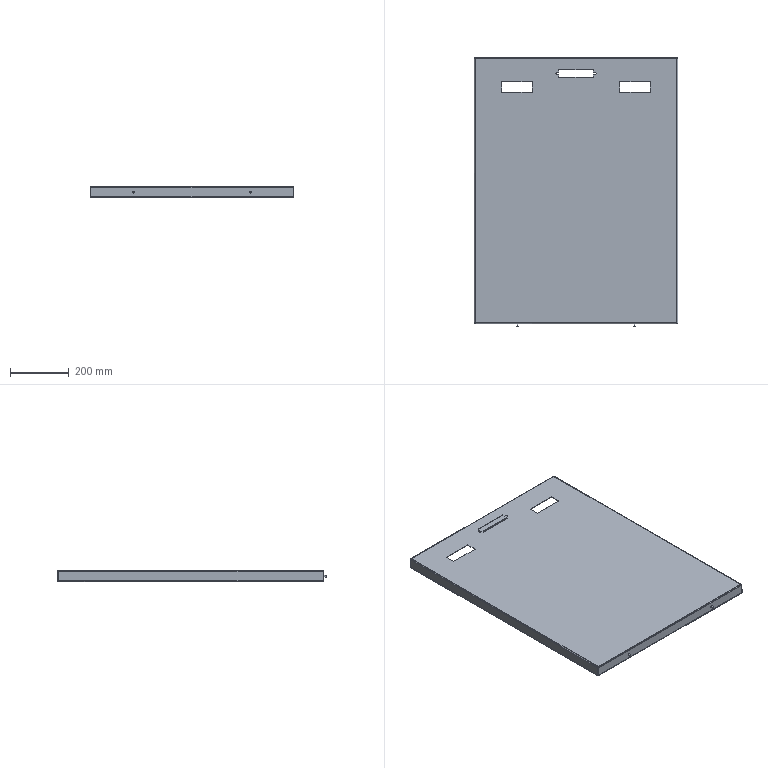Part | SolidWorks | features ICE 6, SMWeldBead 4, EdgeFlange 2, FlatPattern 1, SMBaseFlange 1, SheetMetal 1 | 1 solid | 145 faces | box 695 x 917 x 38 mm | volume 1204871 mm3 | plane 76 | spline 40 | cylinder 29 | commonest cylinder face diameters 4 x8 7 x8 6 x6 2 x4 9 x3